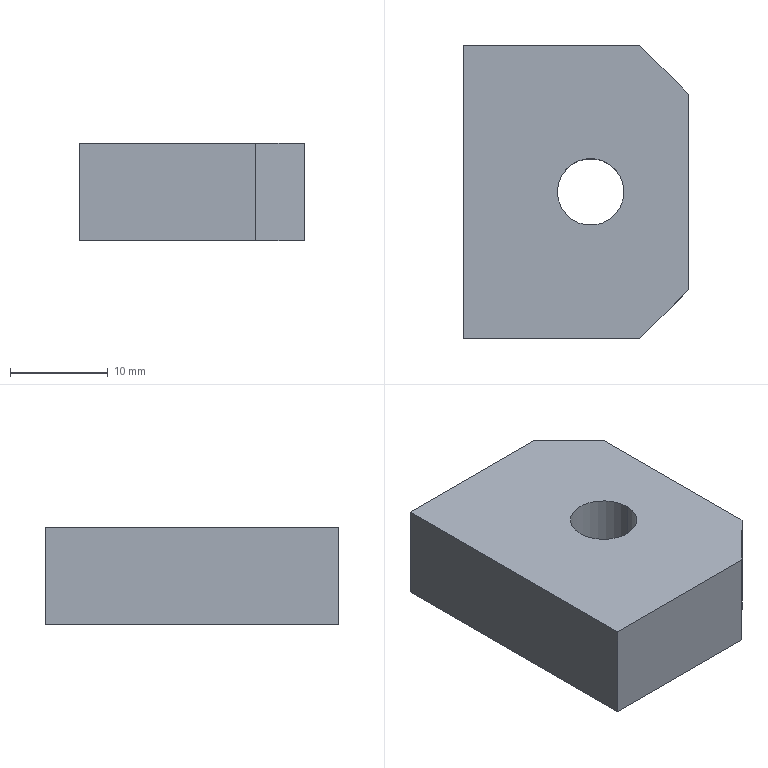Part | SolidWorks | features Chamfer 1, Extrusion 1, HoleWzd 1 | 1 solid | 10 faces | box 23 x 30 x 10 mm | volume 6287 mm3 | plane 8 | cylinder 2 | commonest cylinder face diameters 6.8 x2
STEP:
#1=CARTESIAN_POINT('',(-1.9,0.,10.));
#2=VERTEX_POINT('',#1);
#3=CARTESIAN_POINT('',(4.9,0.,10.));
#4=VERTEX_POINT('',#3);
#5=CARTESIAN_POINT('',(1.5,0.,10.));
#6=DIRECTION('',(0.,0.,1.));
#7=DIRECTION('',(1.,0.,0.));
#8=AXIS2_PLACEMENT_3D('',#5,#6,#7);
#9=CIRCLE('',#8,3.4);
#10=EDGE_CURVE('',#2,#4,#9,.T.);
#11=ORIENTED_EDGE('',*,*,#10,.T.);
#12=CARTESIAN_POINT('',(4.9,0.,0.));
#13=VERTEX_POINT('',#12);
#14=CARTESIAN_POINT('',(4.9,0.,0.));
#15=DIRECTION('',(0.,0.,-1.));
#16=VECTOR('',#15,1000.);
#17=LINE('',#14,#16);
#18=EDGE_CURVE('',#4,#13,#17,.T.);
#19=ORIENTED_EDGE('',*,*,#18,.T.);
#20=CARTESIAN_POINT('',(-1.9,0.,0.));
#21=VERTEX_POINT('',#20);
#22=CARTESIAN_POINT('',(1.5,0.,0.));
#23=DIRECTION('',(0.,0.,-1.));
#24=DIRECTION('',(-1.,0.,0.));
#25=AXIS2_PLACEMENT_3D('',#22,#23,#24);
#26=CIRCLE('',#25,3.4);
#27=EDGE_CURVE('',#13,#21,#26,.T.);
#28=ORIENTED_EDGE('',*,*,#27,.T.);
#29=CARTESIAN_POINT('',(-1.9,0.,0.));
#30=DIRECTION('',(0.,0.,-1.));
#31=VECTOR('',#30,1000.);
#32=LINE('',#29,#31);
#33=EDGE_CURVE('',#2,#21,#32,.T.);
#34=ORIENTED_EDGE('',*,*,#33,.F.);
#35=EDGE_LOOP('',(#11,#19,#28,#34));
#36=FACE_OUTER_BOUND('',#35,.T.);
#37=CARTESIAN_POINT('',(1.5,0.,0.));
#38=DIRECTION('',(0.,0.,-1.));
#39=DIRECTION('',(-1.,0.,0.));
#40=AXIS2_PLACEMENT_3D('',#37,#38,#39);
#41=CYLINDRICAL_SURFACE('',#40,3.4);
#42=ADVANCED_FACE('',(#36),#41,.F.);
#43=CARTESIAN_POINT('',(-11.5,15.,0.));
#44=VERTEX_POINT('',#43);
#45=CARTESIAN_POINT('',(-11.5,-15.,0.));
#46=VERTEX_POINT('',#45);
#47=CARTESIAN_POINT('',(-11.5,-15.,0.));
#48=DIRECTION('',(0.,-1.,0.));
#49=VECTOR('',#48,1000.);
#50=LINE('',#47,#49);
#51=EDGE_CURVE('',#44,#46,#50,.T.);
#52=ORIENTED_EDGE('',*,*,#51,.T.);
#53=CARTESIAN_POINT('',(-11.5,-15.,10.));
#54=VERTEX_POINT('',#53);
#55=CARTESIAN_POINT('',(-11.5,-15.,10.));
#56=DIRECTION('',(0.,0.,-1.));
#57=VECTOR('',#56,1000.);
#58=LINE('',#55,#57);
#59=EDGE_CURVE('',#54,#46,#58,.T.);
#60=ORIENTED_EDGE('',*,*,#59,.F.);
#61=CARTESIAN_POINT('',(-11.5,15.,10.));
#62=VERTEX_POINT('',#61);
#63=CARTESIAN_POINT('',(-11.5,-15.,10.));
#64=DIRECTION('',(0.,-1.,0.));
#65=VECTOR('',#64,1000.);
#66=LINE('',#63,#65);
#67=EDGE_CURVE('',#62,#54,#66,.T.);
#68=ORIENTED_EDGE('',*,*,#67,.F.);
#69=CARTESIAN_POINT('',(-11.5,15.,10.));
#70=DIRECTION('',(0.,0.,-1.));
#71=VECTOR('',#70,1000.);
#72=LINE('',#69,#71);
#73=EDGE_CURVE('',#62,#44,#72,.T.);
#74=ORIENTED_EDGE('',*,*,#73,.T.);
#75=EDGE_LOOP('',(#52,#60,#68,#74));
#76=FACE_OUTER_BOUND('',#75,.T.);
#77=CARTESIAN_POINT('',(-11.5,-15.,10.));
#78=DIRECTION('',(1.,0.,0.));
#79=DIRECTION('',(0.,0.,-1.));
#80=AXIS2_PLACEMENT_3D('',#77,#78,#79);
#81=PLANE('',#80);
#82=ADVANCED_FACE('',(#76),#81,.F.);
#83=CARTESIAN_POINT('',(6.5,-15.,0.));
#84=VERTEX_POINT('',#83);
#85=CARTESIAN_POINT('',(11.5,-15.,0.));
#86=DIRECTION('',(1.,0.,0.));
#87=VECTOR('',#86,1000.);
#88=LINE('',#85,#87);
#89=EDGE_CURVE('',#46,#84,#88,.T.);
#90=ORIENTED_EDGE('',*,*,#89,.T.);
#91=CARTESIAN_POINT('',(6.5,-15.,10.));
#92=VERTEX_POINT('',#91);
#93=CARTESIAN_POINT('',(6.5,-15.,10.));
#94=DIRECTION('',(0.,0.,1.));
#95=VECTOR('',#94,1000.);
#96=LINE('',#93,#95);
#97=EDGE_CURVE('',#84,#92,#96,.T.);
#98=ORIENTED_EDGE('',*,*,#97,.T.);
#99=CARTESIAN_POINT('',(11.5,-15.,10.));
#100=DIRECTION('',(1.,0.,0.));
#101=VECTOR('',#100,1000.);
#102=LINE('',#99,#101);
#103=EDGE_CURVE('',#54,#92,#102,.T.);
#104=ORIENTED_EDGE('',*,*,#103,.F.);
#105=ORIENTED_EDGE('',*,*,#59,.T.);
#106=EDGE_LOOP('',(#90,#98,#104,#105));
#107=FACE_OUTER_BOUND('',#106,.T.);
#108=CARTESIAN_POINT('',(11.5,-15.,10.));
#109=DIRECTION('',(0.,1.,0.));
#110=DIRECTION('',(-1.,0.,0.));
#111=AXIS2_PLACEMENT_3D('',#108,#109,#110);
#112=PLANE('',#111);
#113=ADVANCED_FACE('',(#107),#112,.F.);
#114=CARTESIAN_POINT('',(11.5,-10.,10.));
#115=VERTEX_POINT('',#114);
#116=CARTESIAN_POINT('',(11.5,10.,10.));
#117=VERTEX_POINT('',#116);
#118=CARTESIAN_POINT('',(11.5,-15.,10.));
#119=DIRECTION('',(0.,1.,0.));
#120=VECTOR('',#119,1000.);
#121=LINE('',#118,#120);
#122=EDGE_CURVE('',#115,#117,#121,.T.);
#123=ORIENTED_EDGE('',*,*,#122,.F.);
#124=CARTESIAN_POINT('',(11.5,-10.,0.));
#125=VERTEX_POINT('',#124);
#126=CARTESIAN_POINT('',(11.5,-10.,10.));
#127=DIRECTION('',(0.,0.,-1.));
#128=VECTOR('',#127,1000.);
#129=LINE('',#126,#128);
#130=EDGE_CURVE('',#115,#125,#129,.T.);
#131=ORIENTED_EDGE('',*,*,#130,.T.);
#132=CARTESIAN_POINT('',(11.5,10.,0.));
#133=VERTEX_POINT('',#132);
#134=CARTESIAN_POINT('',(11.5,-15.,0.));
#135=DIRECTION('',(0.,1.,0.));
#136=VECTOR('',#135,1000.);
#137=LINE('',#134,#136);
#138=EDGE_CURVE('',#125,#133,#137,.T.);
#139=ORIENTED_EDGE('',*,*,#138,.T.);
#140=CARTESIAN_POINT('',(11.5,10.,10.));
#141=DIRECTION('',(0.,0.,1.));
#142=VECTOR('',#141,1000.);
#143=LINE('',#140,#142);
#144=EDGE_CURVE('',#133,#117,#143,.T.);
#145=ORIENTED_EDGE('',*,*,#144,.T.);
#146=EDGE_LOOP('',(#123,#131,#139,#145));
#147=FACE_OUTER_BOUND('',#146,.T.);
#148=CARTESIAN_POINT('',(11.5,-15.,10.));
#149=DIRECTION('',(-1.,0.,0.));
#150=DIRECTION('',(0.,0.,1.));
#151=AXIS2_PLACEMENT_3D('',#148,#149,#150);
#152=PLANE('',#151);
#153=ADVANCED_FACE('',(#147),#152,.F.);
#154=CARTESIAN_POINT('',(6.5,15.,10.));
#155=VERTEX_POINT('',#154);
#156=CARTESIAN_POINT('',(11.5,15.,10.));
#157=DIRECTION('',(-1.,0.,0.));
#158=VECTOR('',#157,1000.);
#159=LINE('',#156,#158);
#160=EDGE_CURVE('',#155,#62,#159,.T.);
#161=ORIENTED_EDGE('',*,*,#160,.F.);
#162=CARTESIAN_POINT('',(6.5,15.,0.));
#163=VERTEX_POINT('',#162);
#164=CARTESIAN_POINT('',(6.5,15.,10.));
#165=DIRECTION('',(0.,0.,-1.));
#166=VECTOR('',#165,1000.);
#167=LINE('',#164,#166);
#168=EDGE_CURVE('',#155,#163,#167,.T.);
#169=ORIENTED_EDGE('',*,*,#168,.T.);
#170=CARTESIAN_POINT('',(11.5,15.,0.));
#171=DIRECTION('',(-1.,0.,0.));
#172=VECTOR('',#171,1000.);
#173=LINE('',#170,#172);
#174=EDGE_CURVE('',#163,#44,#173,.T.);
#175=ORIENTED_EDGE('',*,*,#174,.T.);
#176=ORIENTED_EDGE('',*,*,#73,.F.);
#177=EDGE_LOOP('',(#161,#169,#175,#176));
#178=FACE_OUTER_BOUND('',#177,.T.);
#179=CARTESIAN_POINT('',(11.5,15.,10.));
#180=DIRECTION('',(0.,-1.,0.));
#181=DIRECTION('',(1.,0.,0.));
#182=AXIS2_PLACEMENT_3D('',#179,#180,#181);
#183=PLANE('',#182);
#184=ADVANCED_FACE('',(#178),#183,.F.);
#185=ORIENTED_EDGE('',*,*,#10,.F.);
#186=CARTESIAN_POINT('',(1.5,0.,10.));
#187=DIRECTION('',(0.,0.,1.));
#188=DIRECTION('',(1.,0.,0.));
#189=AXIS2_PLACEMENT_3D('',#186,#187,#188);
#190=CIRCLE('',#189,3.4);
#191=EDGE_CURVE('',#4,#2,#190,.T.);
#192=ORIENTED_EDGE('',*,*,#191,.F.);
#193=EDGE_LOOP('',(#185,#192));
#194=FACE_BOUND('',#193,.T.);
#195=ORIENTED_EDGE('',*,*,#103,.T.);
#196=CARTESIAN_POINT('',(10.75,-10.75,10.));
#197=DIRECTION('',(0.7071,0.7071,0.));
#198=VECTOR('',#197,1000.);
#199=LINE('',#196,#198);
#200=EDGE_CURVE('',#92,#115,#199,.T.);
#201=ORIENTED_EDGE('',*,*,#200,.T.);
#202=ORIENTED_EDGE('',*,*,#122,.T.);
#203=CARTESIAN_POINT('',(10.75,10.75,10.));
#204=DIRECTION('',(-0.7071,0.7071,0.));
#205=VECTOR('',#204,1000.);
#206=LINE('',#203,#205);
#207=EDGE_CURVE('',#117,#155,#206,.T.);
#208=ORIENTED_EDGE('',*,*,#207,.T.);
#209=ORIENTED_EDGE('',*,*,#160,.T.);
#210=ORIENTED_EDGE('',*,*,#67,.T.);
#211=EDGE_LOOP('',(#195,#201,#202,#208,#209,#210));
#212=FACE_OUTER_BOUND('',#211,.T.);
#213=CARTESIAN_POINT('',(0.,0.,10.));
#214=DIRECTION('',(0.,0.,1.));
#215=DIRECTION('',(1.,0.,0.));
#216=AXIS2_PLACEMENT_3D('',#213,#214,#215);
#217=PLANE('',#216);
#218=ADVANCED_FACE('',(#194,#212),#217,.T.);
#219=CARTESIAN_POINT('',(1.5,0.,0.));
#220=DIRECTION('',(0.,0.,-1.));
#221=DIRECTION('',(-1.,0.,0.));
#222=AXIS2_PLACEMENT_3D('',#219,#220,#221);
#223=CIRCLE('',#222,3.4);
#224=EDGE_CURVE('',#21,#13,#223,.T.);
#225=ORIENTED_EDGE('',*,*,#224,.F.);
#226=ORIENTED_EDGE('',*,*,#27,.F.);
#227=EDGE_LOOP('',(#225,#226));
#228=FACE_BOUND('',#227,.T.);
#229=ORIENTED_EDGE('',*,*,#138,.F.);
#230=CARTESIAN_POINT('',(11.5,-10.,0.));
#231=DIRECTION('',(-0.7071,-0.7071,0.));
#232=VECTOR('',#231,1000.);
#233=LINE('',#230,#232);
#234=EDGE_CURVE('',#125,#84,#233,.T.);
#235=ORIENTED_EDGE('',*,*,#234,.T.);
#236=ORIENTED_EDGE('',*,*,#89,.F.);
#237=ORIENTED_EDGE('',*,*,#51,.F.);
#238=ORIENTED_EDGE('',*,*,#174,.F.);
#239=CARTESIAN_POINT('',(6.5,15.,0.));
#240=DIRECTION('',(0.7071,-0.7071,0.));
#241=VECTOR('',#240,1000.);
#242=LINE('',#239,#241);
#243=EDGE_CURVE('',#163,#133,#242,.T.);
#244=ORIENTED_EDGE('',*,*,#243,.T.);
#245=EDGE_LOOP('',(#229,#235,#236,#237,#238,#244));
#246=FACE_OUTER_BOUND('',#245,.T.);
#247=CARTESIAN_POINT('',(0.,0.,0.));
#248=DIRECTION('',(0.,0.,1.));
#249=DIRECTION('',(1.,0.,0.));
#250=AXIS2_PLACEMENT_3D('',#247,#248,#249);
#251=PLANE('',#250);
#252=ADVANCED_FACE('',(#228,#246),#251,.F.);
#253=ORIENTED_EDGE('',*,*,#200,.F.);
#254=ORIENTED_EDGE('',*,*,#97,.F.);
#255=ORIENTED_EDGE('',*,*,#234,.F.);
#256=ORIENTED_EDGE('',*,*,#130,.F.);
#257=EDGE_LOOP('',(#253,#254,#255,#256));
#258=FACE_OUTER_BOUND('',#257,.T.);
#259=CARTESIAN_POINT('',(11.5,-10.,10.));
#260=DIRECTION('',(-0.7071,0.7071,0.));
#261=DIRECTION('',(0.,0.,-1.));
#262=AXIS2_PLACEMENT_3D('',#259,#260,#261);
#263=PLANE('',#262);
#264=ADVANCED_FACE('',(#258),#263,.F.);
#265=ORIENTED_EDGE('',*,*,#207,.F.);
#266=ORIENTED_EDGE('',*,*,#144,.F.);
#267=ORIENTED_EDGE('',*,*,#243,.F.);
#268=ORIENTED_EDGE('',*,*,#168,.F.);
#269=EDGE_LOOP('',(#265,#266,#267,#268));
#270=FACE_OUTER_BOUND('',#269,.T.);
#271=CARTESIAN_POINT('',(6.5,15.,10.));
#272=DIRECTION('',(-0.7071,-0.7071,0.));
#273=DIRECTION('',(0.,0.,-1.));
#274=AXIS2_PLACEMENT_3D('',#271,#272,#273);
#275=PLANE('',#274);
#276=ADVANCED_FACE('',(#270),#275,.F.);
#277=ORIENTED_EDGE('',*,*,#18,.F.);
#278=ORIENTED_EDGE('',*,*,#191,.T.);
#279=ORIENTED_EDGE('',*,*,#33,.T.);
#280=ORIENTED_EDGE('',*,*,#224,.T.);
#281=EDGE_LOOP('',(#277,#278,#279,#280));
#282=FACE_OUTER_BOUND('',#281,.T.);
#283=CARTESIAN_POINT('',(1.5,0.,0.));
#284=DIRECTION('',(0.,0.,-1.));
#285=DIRECTION('',(-1.,0.,0.));
#286=AXIS2_PLACEMENT_3D('',#283,#284,#285);
#287=CYLINDRICAL_SURFACE('',#286,3.4);
#288=ADVANCED_FACE('',(#282),#287,.F.);
#289=CLOSED_SHELL('',(#42,#82,#113,#153,#184,#218,#252,#264,#276,#288));
#290=MANIFOLD_SOLID_BREP('',#289);
#291=CARTESIAN_POINT('',(0.,0.,0.));
#292=DIRECTION('',(0.,0.,1.));
#293=DIRECTION('',(1.,0.,0.));
#294=AXIS2_PLACEMENT_3D('',#291,#292,#293);
#295=(LENGTH_UNIT()NAMED_UNIT(*)SI_UNIT(.MILLI.,.METRE.));
#296=UNCERTAINTY_MEASURE_WITH_UNIT(LENGTH_MEASURE(0.00001),#295,'','');
#297=(NAMED_UNIT(*)PLANE_ANGLE_UNIT()SI_UNIT($,.RADIAN.));
#298=(NAMED_UNIT(*)SI_UNIT($,.STERADIAN.)SOLID_ANGLE_UNIT());
#299=(GEOMETRIC_REPRESENTATION_CONTEXT(3)GLOBAL_UNCERTAINTY_ASSIGNED_CONTEXT((#296))GLOBAL_UNIT_ASSIGNED_CONTEXT((#295,#297,#298))REPRESENTATION_CONTEXT('',''));
#300=ADVANCED_BREP_SHAPE_REPRESENTATION('',(#290,#294),#299);